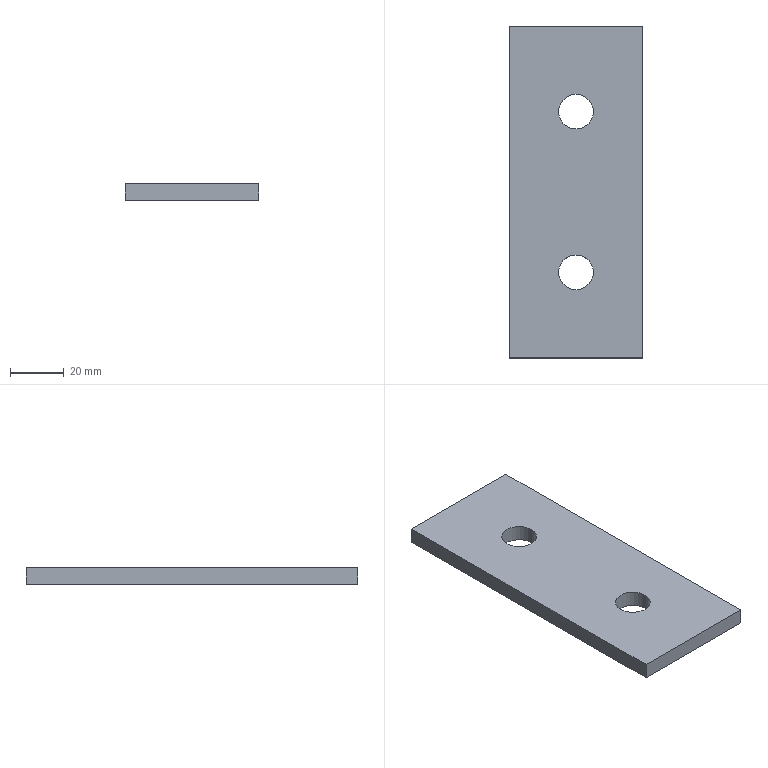Part | SolidWorks | features Extrusion 1, ICE 1 | 1 solid | 10 faces | box 50 x 124 x 6 mm | volume 35607 mm3 | plane 6 | cylinder 4 | commonest cylinder face diameters 13 x4
STEP:
#1=CARTESIAN_POINT('',(-6.5,-30.,-3.));
#2=VERTEX_POINT('',#1);
#3=CARTESIAN_POINT('',(6.5,-30.,-3.));
#4=VERTEX_POINT('',#3);
#5=CARTESIAN_POINT('',(0.,-30.,-3.));
#6=DIRECTION('',(0.,0.,1.));
#7=DIRECTION('',(1.,0.,0.));
#8=AXIS2_PLACEMENT_3D('',#5,#6,#7);
#9=CIRCLE('',#8,6.5);
#10=EDGE_CURVE('',#2,#4,#9,.T.);
#11=ORIENTED_EDGE('',*,*,#10,.F.);
#12=CARTESIAN_POINT('',(-6.5,-30.,3.));
#13=VERTEX_POINT('',#12);
#14=CARTESIAN_POINT('',(-6.5,-30.,-19.));
#15=DIRECTION('',(0.,0.,1.));
#16=VECTOR('',#15,1000.);
#17=LINE('',#14,#16);
#18=EDGE_CURVE('',#2,#13,#17,.T.);
#19=ORIENTED_EDGE('',*,*,#18,.T.);
#20=CARTESIAN_POINT('',(6.5,-30.,3.));
#21=VERTEX_POINT('',#20);
#22=CARTESIAN_POINT('',(0.,-30.,3.));
#23=DIRECTION('',(0.,0.,1.));
#24=DIRECTION('',(1.,0.,0.));
#25=AXIS2_PLACEMENT_3D('',#22,#23,#24);
#26=CIRCLE('',#25,6.5);
#27=EDGE_CURVE('',#13,#21,#26,.T.);
#28=ORIENTED_EDGE('',*,*,#27,.T.);
#29=CARTESIAN_POINT('',(6.5,-30.,-19.));
#30=DIRECTION('',(0.,0.,1.));
#31=VECTOR('',#30,1000.);
#32=LINE('',#29,#31);
#33=EDGE_CURVE('',#4,#21,#32,.T.);
#34=ORIENTED_EDGE('',*,*,#33,.F.);
#35=EDGE_LOOP('',(#11,#19,#28,#34));
#36=FACE_OUTER_BOUND('',#35,.T.);
#37=CARTESIAN_POINT('',(0.,-30.,-19.));
#38=DIRECTION('',(0.,0.,1.));
#39=DIRECTION('',(1.,0.,0.));
#40=AXIS2_PLACEMENT_3D('',#37,#38,#39);
#41=CYLINDRICAL_SURFACE('',#40,6.5);
#42=ADVANCED_FACE('',(#36),#41,.F.);
#43=CARTESIAN_POINT('',(-6.5,30.,-3.));
#44=VERTEX_POINT('',#43);
#45=CARTESIAN_POINT('',(6.5,30.,-3.));
#46=VERTEX_POINT('',#45);
#47=CARTESIAN_POINT('',(0.,30.,-3.));
#48=DIRECTION('',(0.,0.,1.));
#49=DIRECTION('',(1.,0.,0.));
#50=AXIS2_PLACEMENT_3D('',#47,#48,#49);
#51=CIRCLE('',#50,6.5);
#52=EDGE_CURVE('',#44,#46,#51,.T.);
#53=ORIENTED_EDGE('',*,*,#52,.F.);
#54=CARTESIAN_POINT('',(-6.5,30.,3.));
#55=VERTEX_POINT('',#54);
#56=CARTESIAN_POINT('',(-6.5,30.,-19.));
#57=DIRECTION('',(0.,0.,1.));
#58=VECTOR('',#57,1000.);
#59=LINE('',#56,#58);
#60=EDGE_CURVE('',#44,#55,#59,.T.);
#61=ORIENTED_EDGE('',*,*,#60,.T.);
#62=CARTESIAN_POINT('',(6.5,30.,3.));
#63=VERTEX_POINT('',#62);
#64=CARTESIAN_POINT('',(0.,30.,3.));
#65=DIRECTION('',(0.,0.,1.));
#66=DIRECTION('',(1.,0.,0.));
#67=AXIS2_PLACEMENT_3D('',#64,#65,#66);
#68=CIRCLE('',#67,6.5);
#69=EDGE_CURVE('',#55,#63,#68,.T.);
#70=ORIENTED_EDGE('',*,*,#69,.T.);
#71=CARTESIAN_POINT('',(6.5,30.,-19.));
#72=DIRECTION('',(0.,0.,1.));
#73=VECTOR('',#72,1000.);
#74=LINE('',#71,#73);
#75=EDGE_CURVE('',#46,#63,#74,.T.);
#76=ORIENTED_EDGE('',*,*,#75,.F.);
#77=EDGE_LOOP('',(#53,#61,#70,#76));
#78=FACE_OUTER_BOUND('',#77,.T.);
#79=CARTESIAN_POINT('',(0.,30.,-19.));
#80=DIRECTION('',(0.,0.,1.));
#81=DIRECTION('',(1.,0.,0.));
#82=AXIS2_PLACEMENT_3D('',#79,#80,#81);
#83=CYLINDRICAL_SURFACE('',#82,6.5);
#84=ADVANCED_FACE('',(#78),#83,.F.);
#85=CARTESIAN_POINT('',(-25.,-62.,-3.));
#86=VERTEX_POINT('',#85);
#87=CARTESIAN_POINT('',(25.,-62.,-3.));
#88=VERTEX_POINT('',#87);
#89=CARTESIAN_POINT('',(-25.,-62.,-3.));
#90=DIRECTION('',(1.,0.,0.));
#91=VECTOR('',#90,1000.);
#92=LINE('',#89,#91);
#93=EDGE_CURVE('',#86,#88,#92,.T.);
#94=ORIENTED_EDGE('',*,*,#93,.T.);
#95=CARTESIAN_POINT('',(25.,-62.,3.));
#96=VERTEX_POINT('',#95);
#97=CARTESIAN_POINT('',(25.,-62.,3.));
#98=DIRECTION('',(0.,0.,-1.));
#99=VECTOR('',#98,1000.);
#100=LINE('',#97,#99);
#101=EDGE_CURVE('',#96,#88,#100,.T.);
#102=ORIENTED_EDGE('',*,*,#101,.F.);
#103=CARTESIAN_POINT('',(-25.,-62.,3.));
#104=VERTEX_POINT('',#103);
#105=CARTESIAN_POINT('',(-25.,-62.,3.));
#106=DIRECTION('',(1.,0.,0.));
#107=VECTOR('',#106,1000.);
#108=LINE('',#105,#107);
#109=EDGE_CURVE('',#104,#96,#108,.T.);
#110=ORIENTED_EDGE('',*,*,#109,.F.);
#111=CARTESIAN_POINT('',(-25.,-62.,3.));
#112=DIRECTION('',(0.,0.,-1.));
#113=VECTOR('',#112,1000.);
#114=LINE('',#111,#113);
#115=EDGE_CURVE('',#104,#86,#114,.T.);
#116=ORIENTED_EDGE('',*,*,#115,.T.);
#117=EDGE_LOOP('',(#94,#102,#110,#116));
#118=FACE_OUTER_BOUND('',#117,.T.);
#119=CARTESIAN_POINT('',(-25.,-62.,3.));
#120=DIRECTION('',(0.,1.,0.));
#121=DIRECTION('',(0.,0.,1.));
#122=AXIS2_PLACEMENT_3D('',#119,#120,#121);
#123=PLANE('',#122);
#124=ADVANCED_FACE('',(#118),#123,.F.);
#125=CARTESIAN_POINT('',(25.,62.,-3.));
#126=VERTEX_POINT('',#125);
#127=CARTESIAN_POINT('',(25.,-62.,-3.));
#128=DIRECTION('',(0.,1.,0.));
#129=VECTOR('',#128,1000.);
#130=LINE('',#127,#129);
#131=EDGE_CURVE('',#88,#126,#130,.T.);
#132=ORIENTED_EDGE('',*,*,#131,.T.);
#133=CARTESIAN_POINT('',(25.,62.,3.));
#134=VERTEX_POINT('',#133);
#135=CARTESIAN_POINT('',(25.,62.,3.));
#136=DIRECTION('',(0.,0.,-1.));
#137=VECTOR('',#136,1000.);
#138=LINE('',#135,#137);
#139=EDGE_CURVE('',#134,#126,#138,.T.);
#140=ORIENTED_EDGE('',*,*,#139,.F.);
#141=CARTESIAN_POINT('',(25.,-62.,3.));
#142=DIRECTION('',(0.,1.,0.));
#143=VECTOR('',#142,1000.);
#144=LINE('',#141,#143);
#145=EDGE_CURVE('',#96,#134,#144,.T.);
#146=ORIENTED_EDGE('',*,*,#145,.F.);
#147=ORIENTED_EDGE('',*,*,#101,.T.);
#148=EDGE_LOOP('',(#132,#140,#146,#147));
#149=FACE_OUTER_BOUND('',#148,.T.);
#150=CARTESIAN_POINT('',(25.,-62.,3.));
#151=DIRECTION('',(-1.,0.,0.));
#152=DIRECTION('',(0.,0.,1.));
#153=AXIS2_PLACEMENT_3D('',#150,#151,#152);
#154=PLANE('',#153);
#155=ADVANCED_FACE('',(#149),#154,.F.);
#156=CARTESIAN_POINT('',(-25.,62.,-3.));
#157=VERTEX_POINT('',#156);
#158=CARTESIAN_POINT('',(25.,62.,-3.));
#159=DIRECTION('',(-1.,0.,0.));
#160=VECTOR('',#159,1000.);
#161=LINE('',#158,#160);
#162=EDGE_CURVE('',#126,#157,#161,.T.);
#163=ORIENTED_EDGE('',*,*,#162,.T.);
#164=CARTESIAN_POINT('',(-25.,62.,3.));
#165=VERTEX_POINT('',#164);
#166=CARTESIAN_POINT('',(-25.,62.,3.));
#167=DIRECTION('',(0.,0.,-1.));
#168=VECTOR('',#167,1000.);
#169=LINE('',#166,#168);
#170=EDGE_CURVE('',#165,#157,#169,.T.);
#171=ORIENTED_EDGE('',*,*,#170,.F.);
#172=CARTESIAN_POINT('',(25.,62.,3.));
#173=DIRECTION('',(-1.,0.,0.));
#174=VECTOR('',#173,1000.);
#175=LINE('',#172,#174);
#176=EDGE_CURVE('',#134,#165,#175,.T.);
#177=ORIENTED_EDGE('',*,*,#176,.F.);
#178=ORIENTED_EDGE('',*,*,#139,.T.);
#179=EDGE_LOOP('',(#163,#171,#177,#178));
#180=FACE_OUTER_BOUND('',#179,.T.);
#181=CARTESIAN_POINT('',(25.,62.,3.));
#182=DIRECTION('',(0.,-1.,0.));
#183=DIRECTION('',(1.,0.,0.));
#184=AXIS2_PLACEMENT_3D('',#181,#182,#183);
#185=PLANE('',#184);
#186=ADVANCED_FACE('',(#180),#185,.F.);
#187=CARTESIAN_POINT('',(-25.,62.,-3.));
#188=DIRECTION('',(0.,-1.,0.));
#189=VECTOR('',#188,1000.);
#190=LINE('',#187,#189);
#191=EDGE_CURVE('',#157,#86,#190,.T.);
#192=ORIENTED_EDGE('',*,*,#191,.T.);
#193=ORIENTED_EDGE('',*,*,#115,.F.);
#194=CARTESIAN_POINT('',(-25.,62.,3.));
#195=DIRECTION('',(0.,-1.,0.));
#196=VECTOR('',#195,1000.);
#197=LINE('',#194,#196);
#198=EDGE_CURVE('',#165,#104,#197,.T.);
#199=ORIENTED_EDGE('',*,*,#198,.F.);
#200=ORIENTED_EDGE('',*,*,#170,.T.);
#201=EDGE_LOOP('',(#192,#193,#199,#200));
#202=FACE_OUTER_BOUND('',#201,.T.);
#203=CARTESIAN_POINT('',(-25.,62.,3.));
#204=DIRECTION('',(1.,0.,0.));
#205=DIRECTION('',(0.,1.,0.));
#206=AXIS2_PLACEMENT_3D('',#203,#204,#205);
#207=PLANE('',#206);
#208=ADVANCED_FACE('',(#202),#207,.F.);
#209=CARTESIAN_POINT('',(0.,-30.,3.));
#210=DIRECTION('',(0.,0.,1.));
#211=DIRECTION('',(1.,0.,0.));
#212=AXIS2_PLACEMENT_3D('',#209,#210,#211);
#213=CIRCLE('',#212,6.5);
#214=EDGE_CURVE('',#21,#13,#213,.T.);
#215=ORIENTED_EDGE('',*,*,#214,.F.);
#216=ORIENTED_EDGE('',*,*,#27,.F.);
#217=EDGE_LOOP('',(#215,#216));
#218=FACE_BOUND('',#217,.T.);
#219=CARTESIAN_POINT('',(0.,30.,3.));
#220=DIRECTION('',(0.,0.,1.));
#221=DIRECTION('',(1.,0.,0.));
#222=AXIS2_PLACEMENT_3D('',#219,#220,#221);
#223=CIRCLE('',#222,6.5);
#224=EDGE_CURVE('',#63,#55,#223,.T.);
#225=ORIENTED_EDGE('',*,*,#224,.F.);
#226=ORIENTED_EDGE('',*,*,#69,.F.);
#227=EDGE_LOOP('',(#225,#226));
#228=FACE_BOUND('',#227,.T.);
#229=ORIENTED_EDGE('',*,*,#109,.T.);
#230=ORIENTED_EDGE('',*,*,#145,.T.);
#231=ORIENTED_EDGE('',*,*,#176,.T.);
#232=ORIENTED_EDGE('',*,*,#198,.T.);
#233=EDGE_LOOP('',(#229,#230,#231,#232));
#234=FACE_OUTER_BOUND('',#233,.T.);
#235=CARTESIAN_POINT('',(25.,-62.,3.));
#236=DIRECTION('',(0.,0.,1.));
#237=DIRECTION('',(1.,0.,0.));
#238=AXIS2_PLACEMENT_3D('',#235,#236,#237);
#239=PLANE('',#238);
#240=ADVANCED_FACE('',(#218,#228,#234),#239,.T.);
#241=CARTESIAN_POINT('',(0.,-30.,-3.));
#242=DIRECTION('',(0.,0.,1.));
#243=DIRECTION('',(1.,0.,0.));
#244=AXIS2_PLACEMENT_3D('',#241,#242,#243);
#245=CIRCLE('',#244,6.5);
#246=EDGE_CURVE('',#4,#2,#245,.T.);
#247=ORIENTED_EDGE('',*,*,#246,.T.);
#248=ORIENTED_EDGE('',*,*,#10,.T.);
#249=EDGE_LOOP('',(#247,#248));
#250=FACE_BOUND('',#249,.T.);
#251=CARTESIAN_POINT('',(0.,30.,-3.));
#252=DIRECTION('',(0.,0.,1.));
#253=DIRECTION('',(1.,0.,0.));
#254=AXIS2_PLACEMENT_3D('',#251,#252,#253);
#255=CIRCLE('',#254,6.5);
#256=EDGE_CURVE('',#46,#44,#255,.T.);
#257=ORIENTED_EDGE('',*,*,#256,.T.);
#258=ORIENTED_EDGE('',*,*,#52,.T.);
#259=EDGE_LOOP('',(#257,#258));
#260=FACE_BOUND('',#259,.T.);
#261=ORIENTED_EDGE('',*,*,#93,.F.);
#262=ORIENTED_EDGE('',*,*,#191,.F.);
#263=ORIENTED_EDGE('',*,*,#162,.F.);
#264=ORIENTED_EDGE('',*,*,#131,.F.);
#265=EDGE_LOOP('',(#261,#262,#263,#264));
#266=FACE_OUTER_BOUND('',#265,.T.);
#267=CARTESIAN_POINT('',(25.,-62.,-3.));
#268=DIRECTION('',(0.,0.,1.));
#269=DIRECTION('',(1.,0.,0.));
#270=AXIS2_PLACEMENT_3D('',#267,#268,#269);
#271=PLANE('',#270);
#272=ADVANCED_FACE('',(#250,#260,#266),#271,.F.);
#273=ORIENTED_EDGE('',*,*,#60,.F.);
#274=ORIENTED_EDGE('',*,*,#256,.F.);
#275=ORIENTED_EDGE('',*,*,#75,.T.);
#276=ORIENTED_EDGE('',*,*,#224,.T.);
#277=EDGE_LOOP('',(#273,#274,#275,#276));
#278=FACE_OUTER_BOUND('',#277,.T.);
#279=CARTESIAN_POINT('',(0.,30.,-19.));
#280=DIRECTION('',(0.,0.,1.));
#281=DIRECTION('',(1.,0.,0.));
#282=AXIS2_PLACEMENT_3D('',#279,#280,#281);
#283=CYLINDRICAL_SURFACE('',#282,6.5);
#284=ADVANCED_FACE('',(#278),#283,.F.);
#285=ORIENTED_EDGE('',*,*,#18,.F.);
#286=ORIENTED_EDGE('',*,*,#246,.F.);
#287=ORIENTED_EDGE('',*,*,#33,.T.);
#288=ORIENTED_EDGE('',*,*,#214,.T.);
#289=EDGE_LOOP('',(#285,#286,#287,#288));
#290=FACE_OUTER_BOUND('',#289,.T.);
#291=CARTESIAN_POINT('',(0.,-30.,-19.));
#292=DIRECTION('',(0.,0.,1.));
#293=DIRECTION('',(1.,0.,0.));
#294=AXIS2_PLACEMENT_3D('',#291,#292,#293);
#295=CYLINDRICAL_SURFACE('',#294,6.5);
#296=ADVANCED_FACE('',(#290),#295,.F.);
#297=CLOSED_SHELL('',(#42,#84,#124,#155,#186,#208,#240,#272,#284,#296));
#298=MANIFOLD_SOLID_BREP('',#297);
#299=CARTESIAN_POINT('',(0.,0.,0.));
#300=DIRECTION('',(0.,0.,1.));
#301=DIRECTION('',(1.,0.,0.));
#302=AXIS2_PLACEMENT_3D('',#299,#300,#301);
#303=(LENGTH_UNIT()NAMED_UNIT(*)SI_UNIT(.MILLI.,.METRE.));
#304=UNCERTAINTY_MEASURE_WITH_UNIT(LENGTH_MEASURE(0.00001),#303,'','');
#305=(NAMED_UNIT(*)PLANE_ANGLE_UNIT()SI_UNIT($,.RADIAN.));
#306=(NAMED_UNIT(*)SI_UNIT($,.STERADIAN.)SOLID_ANGLE_UNIT());
#307=(GEOMETRIC_REPRESENTATION_CONTEXT(3)GLOBAL_UNCERTAINTY_ASSIGNED_CONTEXT((#304))GLOBAL_UNIT_ASSIGNED_CONTEXT((#303,#305,#306))REPRESENTATION_CONTEXT('',''));
#308=ADVANCED_BREP_SHAPE_REPRESENTATION('',(#298,#302),#307);